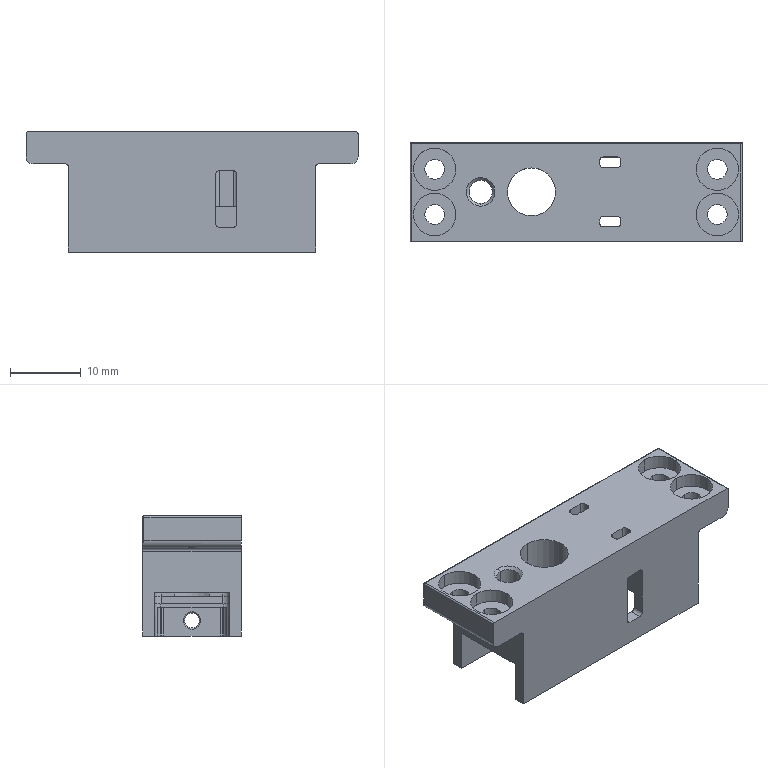NC program | NX | posted with a generic post | part box 47 x 14 x 17 mm
Lines 1 to 1054 of 3166:
N10 G17 G21 G94 G90
(ZLEVEL_PROFILE_COPY_1_COPY_COPY_COPY , TOOL : D2)
N12 T20 M6
N14 G54
N16 G17 G0 G90 X-4.35 Y1.02 B0. C0. S9500 M3
N18 G43 Z30. H20
N20 Z1.
N22 G94 G1 Y4. Z0.844 F1000.
N24 X-5.35 Z0.791
N26 Y-2.001 Z0.477
N28 X-5.308 Y-2. Z0.475
N30 X-4.35 Z0.425
N32 Y4. Z0.11
N34 X-5.35 Z0.058
N36 Y1. Z-0.1
N38 Y-2.001 F850.
N40 X-5.308 Y-2.
N42 X-4.35
N44 Y4.
N46 X-5.35
N48 Y1.
N50 Y-1.951 Z-0.151
N52 Y-2. Z-0.152
N54 X-5.203 Z-0.155
N56 X-4.35 Z-0.169
N58 Y-0.295 Z-0.199
N60 Y4.
N62 X-5.35
N64 Y1.
N66 Y-1.951 Z-0.251
N68 Y-2. Z-0.252
N70 X-5.203 Z-0.254
N72 X-4.35 Z-0.269
N74 Y-0.295 Z-0.299
N76 Y4.
N78 X-5.35
N80 Y1.
N82 Y-1.951 Z-0.35
N84 Y-2. Z-0.351
N86 X-5.203 Z-0.354
N88 X-4.35 Z-0.369
N90 Y-0.295 Z-0.398
N92 Y4.
N94 X-5.35
N96 Y1.
N98 Y-1.951 Z-0.45
N100 Y-2. Z-0.451
N102 X-5.203 Z-0.453
N104 X-4.35 Z-0.468
N106 Y-0.295 Z-0.498
N108 Y4.
N110 X-5.35
N112 Y1.
N114 Y-1.951 Z-0.549
N116 Y-2. Z-0.55
N118 X-5.202 Z-0.553
N120 X-4.35 Z-0.568
N122 Y-0.295 Z-0.598
N124 Y4.
N126 X-5.35
N128 Y1.
N130 Y-1.951 Z-0.649
N132 Y-2. Z-0.65
N134 X-5.202 Z-0.652
N136 X-4.35 Z-0.667
N138 Y-0.295 Z-0.697
N140 Y4.
N142 X-5.35
N144 Y1.
N146 Y-1.951 Z-0.749
N148 Y-2.
N150 X-5.202 Z-0.752
N152 X-4.35 Z-0.767
N154 Y-0.295 Z-0.797
N156 Y4.
N158 X-5.35
N160 Y1.
N162 Y-1.951 Z-0.848
N164 Y-2. Z-0.849
N166 X-5.202 Z-0.852
N168 X-4.35 Z-0.866
N170 Y-0.295 Z-0.896
N172 Y4.
N174 X-5.35
N176 Y1.
N178 Y-1.951 Z-0.948
N180 Y-2. Z-0.949
N182 X-5.202 Z-0.951
N184 X-4.35 Z-0.966
N186 Y-0.295 Z-0.996
N188 Y4.
N190 X-5.35
N192 Y1.
N194 Y-1.951 Z-1.047
N196 Y-2. Z-1.048
N198 X-5.202 Z-1.051
N200 X-4.35 Z-1.066
N202 Y-0.295 Z-1.095
N204 Y4.
N206 X-5.35
N208 Y1.
N210 Y-1.951 Z-1.147
N212 Y-2. Z-1.148
N214 X-5.202 Z-1.15
N216 X-4.35 Z-1.165
N218 Y-0.294 Z-1.195
N220 Y4.
N222 X-5.35
N224 Y1.
N226 Y-2. Z-1.247
N228 X-4.35 Z-1.265
N230 Y-0.294 Z-1.295
N232 Y4.
N234 X-5.35
N236 Y1.
N238 Y-2. Z-1.347
N240 X-4.35 Z-1.364
N242 Y-0.294 Z-1.394
N244 Y4.
N246 X-5.35
N248 Y1.
N250 Y-2. Z-1.447
N252 X-4.35 Z-1.464
N254 Y-0.294 Z-1.494
N256 Y4.
N258 X-5.35
N260 Y1.
N262 Y-2. Z-1.546
N264 X-4.35 Z-1.564
N266 Y-0.294 Z-1.593
N268 Y4.
N270 X-5.35
N272 Y1.
N274 Y-2. Z-1.646
N276 X-4.35 Z-1.663
N278 Y-0.294 Z-1.693
N280 Y4.
N282 X-5.35
N284 Y1.
N286 Y-2. Z-1.745
N288 X-4.35 Z-1.763
N290 Y-0.294 Z-1.793
N292 Y4.
N294 X-5.35
N296 Y1.
N298 Y-2. Z-1.845
N300 X-4.35 Z-1.862
N302 Y-0.294 Z-1.892
N304 Y4.
N306 X-5.35
N308 Y1.
N310 Y-2. Z-1.944
N312 X-4.35 Z-1.962
N314 Y-0.294 Z-1.992
N316 Y4.
N318 X-5.35
N320 Y1.
N322 Y-2. Z-2.044
N324 X-4.35 Z-2.061
N326 Y-0.294 Z-2.091
N328 Y4.
N330 X-5.35
N332 Y1.
N334 Y-2. Z-2.144
N336 X-4.35 Z-2.161
N338 Y-0.294 Z-2.191
N340 Y4.
N342 X-5.35
N344 Y1.
N346 Y-2. Z-2.243
N348 X-4.35 Z-2.261
N350 Y-0.294 Z-2.29
N352 Y4.
N354 X-5.35
N356 Y1.
N358 Y-2. Z-2.343
N360 X-4.35 Z-2.36
N362 Y-0.294 Z-2.39
N364 Y4.
N366 X-5.35
N368 Y1.
N370 Y-2. Z-2.442
N372 X-4.35 Z-2.46
N374 Y-0.294 Z-2.49
N376 Y4.
N378 X-5.35
N380 Y1.
N382 Y-2. Z-2.542
N384 X-4.35 Z-2.559
N386 Y-0.294 Z-2.589
N388 Y4.
N390 X-5.35
N392 Y1.
N394 Y-2. Z-2.642
N396 X-4.35 Z-2.659
N398 Y-0.294 Z-2.689
N400 Y4.
N402 X-5.35
N404 Y1.
N406 Y-2. Z-2.741
N408 X-4.35 Z-2.759
N410 Y-0.294 Z-2.788
N412 Y4.
N414 X-5.35
N416 Y1.
N418 Y-2. Z-2.841
N420 X-4.35 Z-2.858
N422 Y-0.294 Z-2.888
N424 Y4.
N426 X-5.35
N428 Y1.
N430 Y-2. Z-2.94
N432 X-4.35 Z-2.958
N434 Y-0.294 Z-2.988
N436 Y4.
N438 X-5.35
N440 Y1.
N442 Y-2. Z-3.04
N444 X-4.35 Z-3.057
N446 Y-0.294 Z-3.087
N448 Y4.
N450 X-5.35
N452 Y1.
N454 Y-2. Z-3.139
N456 X-4.35 Z-3.157
N458 Y-0.294 Z-3.187
N460 Y4.
N462 X-5.35
N464 Y1.
N466 Y-2. Z-3.239
N468 X-4.35 Z-3.256
N470 Y-0.294 Z-3.286
N472 Y4.
N474 X-5.35
N476 Y1.
N478 Y-2. Z-3.339
N480 X-4.35 Z-3.356
N482 Y-0.294 Z-3.386
N484 Y4.
N486 X-5.35
N488 Y1.
N490 Y-2. Z-3.438
N492 X-4.35 Z-3.456
N494 Y-0.294 Z-3.485
N496 Y4.
N498 X-5.35
N500 Y1.
N502 Y-2. Z-3.538
N504 X-4.35 Z-3.555
N506 Y-0.294 Z-3.585
N508 Y4.
N510 X-5.35
N512 Y1.
N514 Y-2. Z-3.637
N516 X-4.35 Z-3.655
N518 Y-0.294 Z-3.685
N520 Y4.
N522 X-5.35
N524 Y1.
N526 Y-2. Z-3.737
N528 X-4.35 Z-3.754
N530 Y-0.294 Z-3.784
N532 Y4.
N534 X-5.35
N536 Y1.
N538 Y-2. Z-3.837
N540 X-4.35 Z-3.854
N542 Y-0.294 Z-3.884
N544 Y4.
N546 X-5.35
N548 Y1.
N550 Y-2. Z-3.936
N552 X-4.35 Z-3.954
N554 Y-0.294 Z-3.983
N556 Y4.
N558 X-5.35
N560 Y1.
N562 Y-2. Z-4.036
N564 X-4.35 Z-4.053
N566 Y-0.294 Z-4.083
N568 Y4.
N570 X-5.35
N572 Y1.
N574 Y-2. Z-4.135
N576 X-4.35 Z-4.153
N578 Y-0.294 Z-4.183
N580 Y4.
N582 X-5.35
N584 Y1.
N586 Y-2. Z-4.235
N588 X-4.35 Z-4.252
N590 Y-0.294 Z-4.282
N592 Y4.
N594 X-5.35
N596 Y1.
N598 Y-2. Z-4.334
N600 X-4.35 Z-4.352
N602 Y-0.294 Z-4.382
N604 Y4.
N606 X-5.35
N608 Y1.
N610 Y-2. Z-4.434
N612 X-4.35 Z-4.451
N614 Y-0.294 Z-4.481
N616 Y4.
N618 X-5.35
N620 Y1.
N622 Y-2. Z-4.534
N624 X-4.35 Z-4.551
N626 Y-0.294 Z-4.581
N628 Y4.
N630 X-5.35
N632 Y1.
N634 Y-2. Z-4.633
N636 X-4.35 Z-4.651
N638 Y-0.294 Z-4.68
N640 Y4.
N642 X-5.35
N644 Y1.
N646 Y-2. Z-4.733
N648 X-4.35 Z-4.75
N650 Y-0.294 Z-4.78
N652 Y4.
N654 X-5.35
N656 Y1.
N658 Y-2. Z-4.832
N660 X-4.35 Z-4.85
N662 Y-0.294 Z-4.88
N664 Y4.
N666 X-5.35
N668 Y1.
N670 Y-2. Z-4.932
N672 X-4.35 Z-4.949
N674 Y-0.294 Z-4.979
N676 Y4.
N678 X-5.35
N680 Y1.
N682 Y-2. Z-5.032
N684 X-4.35 Z-5.049
N686 Y-0.294 Z-5.079
N688 Y4.
N690 X-5.35
N692 Y1.
N694 Y-2. Z-5.131
N696 X-4.35 Z-5.149
N698 Y-0.294 Z-5.178
N700 Y4.
N702 X-5.35
N704 Y1.
N706 Y-2. Z-5.231
N708 X-4.35 Z-5.248
N710 Y-0.294 Z-5.278
N712 Y4.
N714 X-5.35
N716 Y1.
N718 Y-2. Z-5.33
N720 X-4.35 Z-5.348
N722 Y-0.294 Z-5.378
N724 Y4.
N726 X-5.35
N728 Y1.
N730 Y-2. Z-5.43
N732 X-4.35 Z-5.447
N734 Y-0.294 Z-5.477
N736 Y4.
N738 X-5.35
N740 Y1.
N742 Y-2. Z-5.529
N744 X-4.35 Z-5.547
N746 Y-0.294 Z-5.577
N748 Y4.
N750 X-5.35
N752 Y1.
N754 Y-2. Z-5.629
N756 X-4.35 Z-5.646
N758 Y-0.294 Z-5.676
N760 Y4.
N762 X-5.35
N764 Y1.
N766 Y-2. Z-5.729
N768 X-4.35 Z-5.746
N770 Y-0.294 Z-5.776
N772 Y4.
N774 X-5.35
N776 Y1.
N778 Y-2. Z-5.828
N780 X-4.35 Z-5.846
N782 Y-0.294 Z-5.875
N784 Y4.
N786 X-5.35
N788 Y1.
N790 Y-2. Z-5.928
N792 X-4.35 Z-5.945
N794 Y-0.294 Z-5.975
N796 Y4.
N798 X-5.35
N800 Y1.
N802 Y-2. Z-6.027
N804 X-4.35 Z-6.045
N806 Y-0.294 Z-6.075
N808 Y4.
N810 X-5.35
N812 Y1.
N814 Y-2. Z-6.127
N816 X-4.35 Z-6.144
N818 Y-0.294 Z-6.174
N820 Y4.
N822 X-5.35
N824 Y1.
N826 Y-2. Z-6.227
N828 X-4.35 Z-6.244
N830 Y-0.294 Z-6.274
N832 Y4.
N834 X-5.35
N836 Y1.
N838 Y-2. Z-6.326
N840 X-4.35 Z-6.344
N842 Y-0.294 Z-6.373
N844 Y4.
N846 X-5.35
N848 Y1.
N850 Y-2. Z-6.426
N852 X-4.35 Z-6.443
N854 Y-0.294 Z-6.473
N856 Y4.
N858 X-5.35
N860 Y1.
N862 Y-2. Z-6.525
N864 X-4.35 Z-6.543
N866 Y-0.294 Z-6.573
N868 Y4.
N870 X-5.35
N872 Y1.
N874 Y-2. Z-6.625
N876 X-4.35 Z-6.642
N878 Y-0.294 Z-6.672
N880 Y4.
N882 X-5.35
N884 Y1.
N886 Y-2. Z-6.724
N888 X-4.35 Z-6.742
N890 Y-0.294 Z-6.772
N892 Y4.
N894 X-5.35
N896 Y1.
N898 Y-2. Z-6.824
N900 X-4.35 Z-6.841
N902 Y-0.294 Z-6.871
N904 Y4.
N906 X-5.35
N908 Y1.
N910 Y-2. Z-6.924
N912 X-4.35 Z-6.941
N914 Y-0.294 Z-6.971
N916 Y4.
N918 X-5.35
N920 Y1.
N922 Y-2. Z-7.023
N924 X-4.35 Z-7.041
N926 Y-0.294 Z-7.07
N928 Y4.
N930 X-5.35
N932 Y1.
N934 Y-2. Z-7.123
N936 X-4.35 Z-7.14
N938 Y-0.294 Z-7.17
N940 Y4.
N942 X-5.35
N944 Y1.
N946 Y-2. Z-7.222
N948 X-4.35 Z-7.24
N950 Y-0.294 Z-7.27
N952 Y4.
N954 X-5.35
N956 Y1.
N958 Y-2. Z-7.322
N960 X-4.35 Z-7.339
N962 Y-0.294 Z-7.369
N964 Y4.
N966 X-5.35
N968 Y1.
N970 Y-2. Z-7.422
N972 X-4.35 Z-7.439
N974 Y-0.294 Z-7.469
N976 Y4.
N978 X-5.35
N980 Y1.
N982 Y-2. Z-7.521
N984 X-4.35 Z-7.539
N986 Y-0.294 Z-7.568
N988 Y4.
N990 X-5.35
N992 Y1.
N994 Y-2. Z-7.621
N996 X-4.35 Z-7.638
N998 Y-0.294 Z-7.668
N1000 Y4.
N1002 X-5.35
N1004 Y1.
N1006 Y-2. Z-7.72
N1008 X-4.35 Z-7.738
N1010 Y-0.294 Z-7.768
N1012 Y4.
N1014 X-5.35
N1016 Y1.
N1018 Y-2. Z-7.82
N1020 X-4.35 Z-7.837
N1022 Y-0.294 Z-7.867
N1024 Y4.
N1026 X-5.35
N1028 Y1.
N1030 Y-2. Z-7.919
N1032 X-4.35 Z-7.937
N1034 Y-0.294 Z-7.967
N1036 Y4.
N1038 X-5.35
N1040 Y1.
N1042 Y-2. Z-8.019
N1044 X-4.35 Z-8.036
N1046 Y-0.294 Z-8.066
N1048 Y4.
N1050 X-5.35
N1052 Y1.
N1054 Y-2. Z-8.119
N1056 X-4.35 Z-8.136
N1058 Y-0.294 Z-8.166
N1060 Y4.
N1062 X-5.35
N1064 Y1.
N1066 Y-2. Z-8.218
N1068 X-4.35 Z-8.236
N1070 Y-0.294 Z-8.265
N1072 Y4.
N1074 X-5.35
N1076 Y1.
N1078 Y-2. Z-8.318
N1080 X-4.35 Z-8.335
N1082 Y-0.294 Z-8.365
N1084 Y4.
N1086 X-5.35
N1088 Y1.
N1090 Y-2. Z-8.417
N1092 X-4.35 Z-8.435
N1094 Y-0.294 Z-8.465
N1096 Y4.
N1098 X-5.35
N1100 Y1.
N1102 Y-2. Z-8.517
N1104 X-4.35 Z-8.534
N1106 Y-0.294 Z-8.564
N1108 Y4.
N1110 X-5.35
N1112 Y1.
N1114 Y-2. Z-8.617
N1116 X-4.35 Z-8.634
N1118 Y-0.294 Z-8.664
N1120 Y4.
N1122 X-5.35
N1124 Y1.
N1126 Y-2. Z-8.716
N1128 X-4.35 Z-8.734
N1130 Y-0.294 Z-8.763
N1132 Y4.
N1134 X-5.35
N1136 Y1.
N1138 Y-2. Z-8.816
N1140 X-4.35 Z-8.833
N1142 Y-0.294 Z-8.863
N1144 Y4.
N1146 X-5.35
N1148 Y1.
N1150 Y-2. Z-8.915
N1152 X-4.35 Z-8.933
N1154 Y-0.294 Z-8.963
N1156 Y4.
N1158 X-5.35
N1160 Y1.
N1162 Y-2. Z-9.015
N1164 X-4.35 Z-9.032
N1166 Y-0.294 Z-9.062
N1168 Y4.
N1170 X-5.35
N1172 Y1.
N1174 Y-2. Z-9.114
N1176 X-4.35 Z-9.132
N1178 Y-0.294 Z-9.162
N1180 Y4.
N1182 X-5.35
N1184 Y1.
N1186 Y-2. Z-9.214
N1188 X-4.35 Z-9.231
N1190 Y-0.294 Z-9.261
N1192 Y4.
N1194 X-5.35
N1196 Y1.
N1198 Y-2. Z-9.314
N1200 X-4.35 Z-9.331
N1202 Y-0.294 Z-9.361
N1204 Y4.
N1206 X-5.35
N1208 Y1.
N1210 Y-2. Z-9.413
N1212 X-4.35 Z-9.431
N1214 Y-0.294 Z-9.46
N1216 Y4.
N1218 X-5.35
N1220 Y1.
N1222 Y-2. Z-9.513
N1224 X-4.35 Z-9.53
N1226 Y-0.294 Z-9.56
N1228 Y4.
N1230 X-5.35
N1232 Y1.
N1234 Y-2. Z-9.612
N1236 X-4.35 Z-9.63
N1238 Y-0.294 Z-9.66
N1240 Y4.
N1242 X-5.35
N1244 Y1.
N1246 Y-2. Z-9.712
N1248 X-4.35 Z-9.729
N1250 Y-0.294 Z-9.759
N1252 Y4.
N1254 X-5.35
N1256 Y1.
N1258 Y-2. Z-9.812
N1260 X-4.35 Z-9.829
N1262 Y-0.294 Z-9.859
N1264 Y4.
N1266 X-5.35
N1268 Y1.
N1270 Y-2. Z-9.911
N1272 X-4.35 Z-9.929
N1274 Y-0.294 Z-9.958
N1276 Y4.
N1278 X-5.35
N1280 Y1.
N1282 Y-2. Z-10.011
N1284 X-4.35 Z-10.028
N1286 Y-0.294 Z-10.058
N1288 Y4.
N1290 X-5.35
N1292 Y1.
N1294 Y-2. Z-10.11
N1296 X-4.35 Z-10.128
N1298 Y-0.294 Z-10.158
N1300 Y4.
N1302 X-5.35
N1304 Y1.
N1306 Y-2. Z-10.21
N1308 X-4.35 Z-10.227
N1310 Y-0.294 Z-10.257
N1312 Y4.
N1314 X-5.35
N1316 Y1.
N1318 Y-2. Z-10.309
N1320 X-4.35 Z-10.327
N1322 Y-0.294 Z-10.357
N1324 Y4.
N1326 X-5.35
N1328 Y1.
N1330 Y-2. Z-10.409
N1332 X-4.35 Z-10.426
N1334 Y-0.294 Z-10.456
N1336 Y4.
N1338 X-5.35
N1340 Y1.
N1342 Y-2. Z-10.509
N1344 X-4.35 Z-10.526
N1346 Y-0.294 Z-10.556
N1348 Y4.
N1350 X-5.35
N1352 Y1.
N1354 Y-2. Z-10.608
N1356 X-4.35 Z-10.626
N1358 Y-0.294 Z-10.655
N1360 Y4.
N1362 X-5.35
N1364 Y1.
N1366 Y-2. Z-10.708
N1368 X-4.35 Z-10.725
N1370 Y-0.294 Z-10.755
N1372 Y4.
N1374 X-5.35
N1376 Y1.
N1378 Y-2. Z-10.807
N1380 X-4.35 Z-10.825
N1382 Y-0.294 Z-10.855
N1384 Y4.
N1386 X-5.35
N1388 Y1.
N1390 Y-2. Z-10.907
N1392 X-4.35 Z-10.924
N1394 Y-0.294 Z-10.954
N1396 Y4.
N1398 X-5.35
N1400 Y1.
N1402 Y-2. Z-11.007
N1404 X-4.35 Z-11.024
N1406 Y-0.294 Z-11.054
N1408 Y4.
N1410 X-5.35
N1412 Y1.
N1414 Y-2. Z-11.106
N1416 X-4.35 Z-11.124
N1418 Y-0.294 Z-11.153
N1420 Y4.
N1422 X-5.35
N1424 Y1.
N1426 Y-1.951 Z-11.205
N1428 Y-2. Z-11.206
N1430 X-5.198 Z-11.208
N1432 X-4.35 Z-11.223
N1434 Y-0.291 Z-11.253
N1436 Y4.
N1438 X-5.35
N1440 Y1.
N1442 Y-1.951 Z-11.304
N1444 Y-2. Z-11.305
N1446 X-5.198 Z-11.308
N1448 X-4.35 Z-11.323
N1450 Y-0.291 Z-11.353
N1452 Y4.
N1454 X-5.35
N1456 Y1.
N1458 Y-1.951 Z-11.404
N1460 Y-2. Z-11.405
N1462 X-5.198 Z-11.407
N1464 X-4.35 Z-11.422
N1466 Y-0.488 Z-11.449
N1468 Y-0.389 Z-11.45
N1470 Y-0.291 Z-11.452
N1472 Y4.
N1474 X-5.35
N1476 Y1.
N1478 Y0.901 Z-11.454
N1480 Y0.803 Z-11.456
N1482 Y0.704 Z-11.457
N1484 Y0.606 Z-11.459
N1486 Y0.508 Z-11.461
N1488 Y0.409 Z-11.462
N1490 Y0.311 Z-11.464
N1492 Y0.213 Z-11.466
N1494 Y0.114 Z-11.468
N1496 Y0.016 Z-11.469
N1498 Y-0.082 Z-11.471
N1500 X-5.349 Y-0.181 Z-11.473
N1502 Y-0.279 Z-11.474
N1504 Y-0.378 Z-11.476
N1506 Y-0.476 Z-11.478
N1508 Y-0.574 Z-11.48
N1510 Y-0.673 Z-11.481
N1512 Y-0.771 Z-11.483
N1514 Y-0.869 Z-11.485
N1516 Y-0.968 Z-11.486
N1518 Y-1.066 Z-11.488
N1520 X-5.348 Y-1.165 Z-11.49
N1522 Y-1.263 Z-11.492
N1524 Y-1.361 Z-11.493
N1526 Y-1.46 Z-11.495
N1528 Y-1.558 Z-11.497
N1530 Y-1.656 Z-11.498
N1532 X-5.347 Y-1.755 Z-11.5
N1534 Y-1.853 Z-11.502
N1536 Y-1.951 Z-11.504
N1538 Y-2.
N1540 X-5.198 Z-11.507
N1542 X-4.411 Z-11.521
N1544 X-4.355 Z-11.522
N1546 X-4.356 Y-1.865 Z-11.524
N1548 Y-1.766 Z-11.526
N1550 Y-1.668 Z-11.528
N1552 Y-1.57 Z-11.529
N1554 X-4.357 Y-1.471 Z-11.531
N1556 Y-1.373 Z-11.533
N1558 Y-1.274 Z-11.534
N1560 Y-1.176 Z-11.536
N1562 X-4.358 Y-1.078 Z-11.538
N1564 Y-0.979 Z-11.54
N1566 Y-0.881 Z-11.541
N1568 X-4.359 Y-0.783 Z-11.543
N1570 Y-0.684 Z-11.545
N1572 Y-0.586 Z-11.547
N1574 X-4.36 Y-0.488 Z-11.548
N1576 Y-0.389 Z-11.55
N1578 Y-0.291 Z-11.552
N1580 Y1.974
N1582 X-4.368 Y1.999
N1584 X-4.358 Y2.124
N1586 X-4.35 Y2.147
N1588 Y4.
N1590 X-5.35
N1592 Y2.147
N1594 X-5.342 Y2.124
N1596 X-5.332 Y1.999
N1598 X-5.34 Y1.974
N1600 Y1.
N1602 X-5.339 Y0.901 Z-11.553
N1604 Y0.803 Z-11.555
N1606 X-5.338 Y0.704 Z-11.557
N1608 Y0.606 Z-11.559
N1610 Y0.508 Z-11.56
N1612 X-5.337 Y0.409 Z-11.562
N1614 Y0.311 Z-11.564
N1616 Y0.213 Z-11.565
N1618 X-5.336 Y0.114 Z-11.567
N1620 Y0.016 Z-11.569
N1622 X-5.335 Y-0.082 Z-11.571
N1624 Y-0.181 Z-11.572
N1626 X-5.334 Y-0.279 Z-11.574
N1628 Y-0.378 Z-11.576
N1630 X-5.333 Y-0.476 Z-11.577
N1632 Y-0.574 Z-11.579
N1634 Y-0.673 Z-11.581
N1636 X-5.332 Y-0.771 Z-11.583
N1638 Y-0.869 Z-11.584
N1640 X-5.331 Y-0.968 Z-11.586
N1642 Y-1.066 Z-11.588
N1644 X-5.33 Y-1.165 Z-11.589
N1646 Y-1.263 Z-11.591
N1648 X-5.329 Y-1.361 Z-11.593
N1650 Y-1.46 Z-11.595
N1652 X-5.328 Y-1.558 Z-11.596
N1654 Y-1.656 Z-11.598
N1656 X-5.327 Y-1.755 Z-11.6
N1658 Y-1.853 Z-11.601
N1660 X-5.326 Y-1.951 Z-11.603
N1662 Y-2. Z-11.604
N1664 X-5.191 Z-11.607
N1666 X-4.38 Z-11.621
N1668 X-4.381 Y-1.847 Z-11.624
N1670 X-4.382 Y-1.749 Z-11.625
N1672 Y-1.651 Z-11.627
N1674 X-4.383 Y-1.552 Z-11.629
N1676 X-4.384 Y-1.454 Z-11.631
N1678 Y-1.356 Z-11.632
N1680 X-4.385 Y-1.257 Z-11.634
N1682 X-4.386 Y-1.159 Z-11.636
N1684 Y-1.06 Z-11.638
N1686 X-4.387 Y-0.962 Z-11.639
N1688 X-4.388 Y-0.864 Z-11.641
N1690 X-4.389 Y-0.765 Z-11.643
N1692 Y-0.667 Z-11.644
N1694 X-4.39 Y-0.569 Z-11.646
N1696 X-4.391 Y-0.47 Z-11.648
N1698 X-4.392 Y-0.372 Z-11.65
N1700 Y-0.273 Z-11.651
N1702 Y2.116
N1704 X-4.397 Y2.179
N1706 X-4.383 Y2.241
N1708 X-4.35 Y2.296
N1710 Y4.
N1712 X-5.35
N1714 Y2.296
N1716 G2 X-5.302 Y2. R0.682
N1718 G1 X-5.308 Y1.985
N1720 Y1.
N1722 X-5.307 Y0.901 Z-11.653
N1724 X-5.306 Y0.803 Z-11.655
N1726 X-5.305 Y0.704 Z-11.656
N1728 Y0.606 Z-11.658
N1730 X-5.304 Y0.508 Z-11.66
N1732 X-5.303 Y0.409 Z-11.662
N1734 X-5.302 Y0.311 Z-11.663
N1736 X-5.301 Y0.213 Z-11.665
N1738 Y0.114 Z-11.667
N1740 X-5.3 Y0.016 Z-11.668
N1742 X-5.299 Y-0.082 Z-11.67
N1744 X-5.298 Y-0.181 Z-11.672
N1746 X-5.297 Y-0.279 Z-11.674
N1748 X-5.296 Y-0.378 Z-11.675
N1750 X-5.295 Y-0.476 Z-11.677
N1752 Y-0.574 Z-11.679
N1754 X-5.294 Y-0.673 Z-11.68
N1756 X-5.293 Y-0.771 Z-11.682
N1758 X-5.292 Y-0.869 Z-11.684
N1760 X-5.291 Y-0.968 Z-11.686
N1762 X-5.29 Y-1.066 Z-11.687
N1764 X-5.289 Y-1.165 Z-11.689
N1766 X-5.288 Y-1.263 Z-11.691
N1768 X-5.287 Y-1.361 Z-11.692
N1770 X-5.286 Y-1.46 Z-11.694
N1772 X-5.285 Y-1.558 Z-11.696
N1774 X-5.284 Y-1.656 Z-11.698
N1776 X-5.283 Y-1.755 Z-11.699
N1778 X-5.282 Y-1.853 Z-11.701
N1780 X-5.281 Y-1.951 Z-11.703
N1782 Y-2. Z-11.704
N1784 X-5.16 Z-11.706
N1786 X-4.569 Z-11.716
N1788 X-4.429 Z-11.72
N1790 X-4.43 Y-1.882 Z-11.722
N1792 X-4.431 Y-1.784 Z-11.723
N1794 X-4.432 Y-1.685 Z-11.725
N1796 X-4.434 Y-1.587 Z-11.727
N1798 X-4.435 Y-1.489 Z-11.729
N1800 X-4.436 Y-1.39 Z-11.73
N1802 X-4.437 Y-1.292 Z-11.732
N1804 X-4.438 Y-1.193 Z-11.734
N1806 X-4.439 Y-1.095 Z-11.735
N1808 X-4.441 Y-0.997 Z-11.737
N1810 X-4.442 Y-0.898 Z-11.739
N1812 X-4.443 Y-0.8 Z-11.741
N1814 X-4.444 Y-0.702 Z-11.742
N1816 X-4.446 Y-0.603 Z-11.744
N1818 X-4.447 Y-0.505 Z-11.746
N1820 X-4.448 Y-0.407 Z-11.747
N1822 X-4.449 Y-0.308 Z-11.749
N1824 X-4.451 Y-0.21 Z-11.751
N1826 Y1.977
N1828 X-4.461 Y1.979
N1830 G2 X-4.35 Y2.458 R0.966
N1832 G1 Y4.
N1834 X-5.35
N1836 Y2.469
N1838 G2 X-5.239 Y1.979 R1.029
N1840 G1 X-5.249 Y1.977
N1842 Y1.
N1844 X-5.248 Y0.901 Z-11.753
N1846 X-5.247 Y0.803 Z-11.754
N1848 X-5.245 Y0.704 Z-11.756
N1850 X-5.244 Y0.606 Z-11.758
N1852 X-5.243 Y0.508 Z-11.759
N1854 X-5.241 Y0.409 Z-11.761
N1856 X-5.24 Y0.311 Z-11.763
N1858 X-5.239 Y0.213 Z-11.765
N1860 X-5.237 Y0.114 Z-11.766
N1862 X-5.236 Y0.016 Z-11.768
N1864 X-5.234 Y-0.082 Z-11.77
N1866 X-5.233 Y-0.181 Z-11.771
N1868 X-5.232 Y-0.279 Z-11.773
N1870 X-5.23 Y-0.378 Z-11.775
N1872 X-5.229 Y-0.476 Z-11.777
N1874 X-5.227 Y-0.574 Z-11.778
N1876 X-5.226 Y-0.673 Z-11.78
N1878 X-5.224 Y-0.771 Z-11.782
N1880 X-5.223 Y-0.869 Z-11.783
N1882 X-5.221 Y-0.968 Z-11.785
N1884 X-5.219 Y-1.066 Z-11.787
N1886 X-5.218 Y-1.165 Z-11.789
N1888 X-5.216 Y-1.263 Z-11.79
N1890 X-5.215 Y-1.361 Z-11.792
N1892 X-5.213 Y-1.46 Z-11.794
N1894 X-5.211 Y-1.558 Z-11.795
N1896 X-5.21 Y-1.656 Z-11.797
N1898 X-5.208 Y-1.755 Z-11.799
N1900 X-5.206 Y-1.853 Z-11.801
N1902 X-5.205 Y-1.951 Z-11.802
N1904 X-5.204 Y-2. Z-11.803
N1906 X-5.101 Z-11.806
N1908 X-4.708 Z-11.813
N1910 X-4.511 Z-11.817
N1912 X-4.513 Y-1.864 Z-11.82
N1914 X-4.515 Y-1.765 Z-11.821
N1916 X-4.517 Y-1.667 Z-11.823
N1918 X-4.519 Y-1.569 Z-11.825
N1920 X-4.521 Y-1.47 Z-11.826
N1922 X-4.523 Y-1.372 Z-11.828
N1924 X-4.525 Y-1.274 Z-11.83
N1926 X-4.527 Y-1.175 Z-11.832
N1928 X-4.529 Y-1.077 Z-11.833
N1930 X-4.531 Y-0.978 Z-11.835
N1932 X-4.533 Y-0.88 Z-11.837
N1934 X-4.535 Y-0.782 Z-11.838
N1936 X-4.537 Y-0.683 Z-11.84
N1938 X-4.539 Y-0.585 Z-11.842
N1940 X-4.542 Y-0.487 Z-11.844
N1942 X-4.544 Y-0.388 Z-11.845
N1944 X-4.546 Y-0.29 Z-11.847
N1946 X-4.548 Y-0.191 Z-11.849
N1948 X-4.551 Y-0.093 Z-11.85
N1950 Y1.957
N1952 X-4.553 Y1.978
N1954 G2 X-4.35 Y2.621 R0.856
N1956 G1 Y4.
N1958 X-5.35
N1960 Y2.652
N1962 G2 X-5.137 Y2.083 R1.19
N1964 G1 X-5.149 Y1.957
N1966 Y1.
N1968 X-5.147 Y0.901 Z-11.852
N1970 X-5.145 Y0.803 Z-11.854
N1972 X-5.142 Y0.704 Z-11.856
N1974 X-5.14 Y0.606 Z-11.857
N1976 X-5.138 Y0.508 Z-11.859
N1978 X-5.135 Y0.409 Z-11.861
N1980 X-5.133 Y0.311 Z-11.862
N1982 X-5.13 Y0.213 Z-11.864
N1984 X-5.128 Y0.114 Z-11.866
N1986 X-5.125 Y0.016 Z-11.868
N1988 X-5.122 Y-0.082 Z-11.869
N1990 X-5.12 Y-0.181 Z-11.871
N1992 X-5.117 Y-0.279 Z-11.873
N1994 X-5.114 Y-0.378 Z-11.874
N1996 X-5.111 Y-0.476 Z-11.876
N1998 X-5.109 Y-0.574 Z-11.878
N2000 X-5.106 Y-0.673 Z-11.88
N2002 X-5.103 Y-0.771 Z-11.881
N2004 X-5.1 Y-0.869 Z-11.883
N2006 X-5.097 Y-0.968 Z-11.885
N2008 X-5.094 Y-1.066 Z-11.886
N2010 X-5.091 Y-1.165 Z-11.888
N2012 X-5.088 Y-1.263 Z-11.89
N2014 X-5.084 Y-1.361 Z-11.892
N2016 X-5.081 Y-1.46 Z-11.893
N2018 X-5.078 Y-1.558 Z-11.895
N2020 X-5.074 Y-1.656 Z-11.897
N2022 X-5.071 Y-1.755 Z-11.898
N2024 X-5.068 Y-1.853 Z-11.9
N2026 X-5.064 Y-1.951 Z-11.902
N2028 X-5.062 Y-2. Z-11.903
N2030 X-4.998 Z-11.904
N2032 X-4.805 Z-11.909
N2034 X-4.661 Z-11.912
N2036 X-4.668 Y-1.861 Z-11.916
N2038 X-4.672 Y-1.762 Z-11.917
N2040 X-4.677 Y-1.664 Z-11.919
N2042 X-4.682 Y-1.565 Z-11.921
N2044 X-4.687 Y-1.467 Z-11.923
N2046 X-4.692 Y-1.369 Z-11.924
N2048 X-4.697 Y-1.27 Z-11.926
N2050 X-4.702 Y-1.172 Z-11.928
N2052 X-4.708 Y-1.074 Z-11.929
N2054 X-4.714 Y-0.975 Z-11.931
N2056 X-4.72 Y-0.877 Z-11.933
N2058 X-4.727 Y-0.779 Z-11.935
N2060 X-4.734 Y-0.68 Z-11.936
N2062 X-4.741 Y-0.582 Z-11.938
N2064 X-4.749 Y-0.483 Z-11.94
N2066 X-4.758 Y-0.385 Z-11.941
N2068 X-4.767 Y-0.287 Z-11.943
N2070 X-4.778 Y-0.188 Z-11.945
N2072 X-4.792 Y-0.09 Z-11.947
N2074 X-4.799 Y-0.041
N2076 X-4.809 Y0.008 Z-11.948
N2078 X-4.8 Y0.058 Z-11.949
N2080 Y0.107 Z-11.95
N2082 Y2.08
N2084 G2 X-4.35 Y2.852 R0.888
N2086 G1 Y4.
N2088 X-5.35
N2090 Y2.842
N2092 G2 X-4.9 Y2.091 R0.851
N2094 G1 Y-2.
N2096 X-4.8
N2098 Y0.107
N2100 G3 X-4.9 Y0.28 R0.2
N2102 G1 Z-11.75
N2104 G0 Z30.
N2106 M5